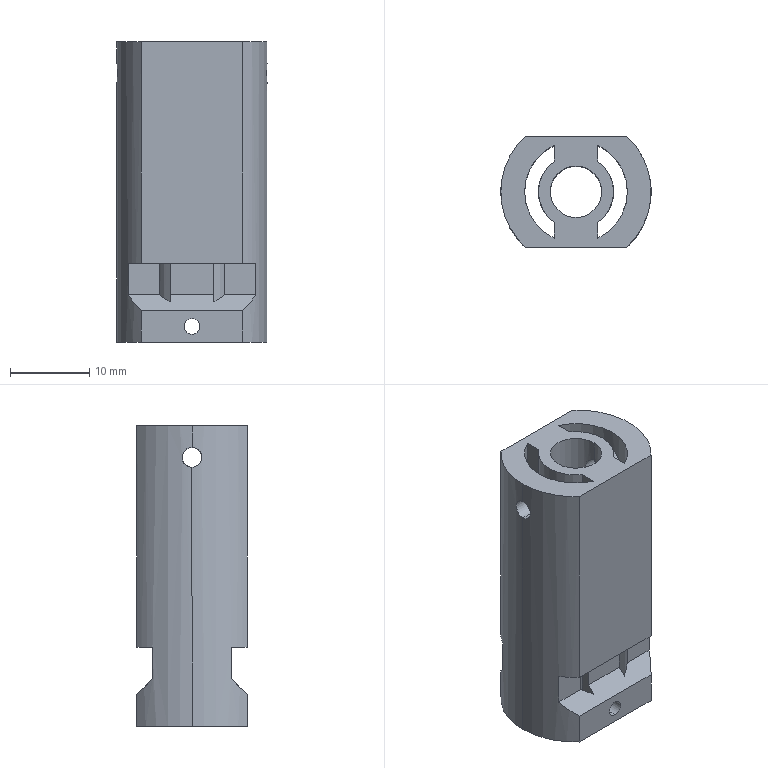Part | STEP file | magnetizing head 1 | 1 solid | 47 faces | box 19 x 14 x 38 mm | volume 5895 mm3 | plane 24 | cylinder 23 | commonest cylinder face diameters 2.5 x8 2 x4 9.5 x3 13 x3 19 x3 6.5 x2